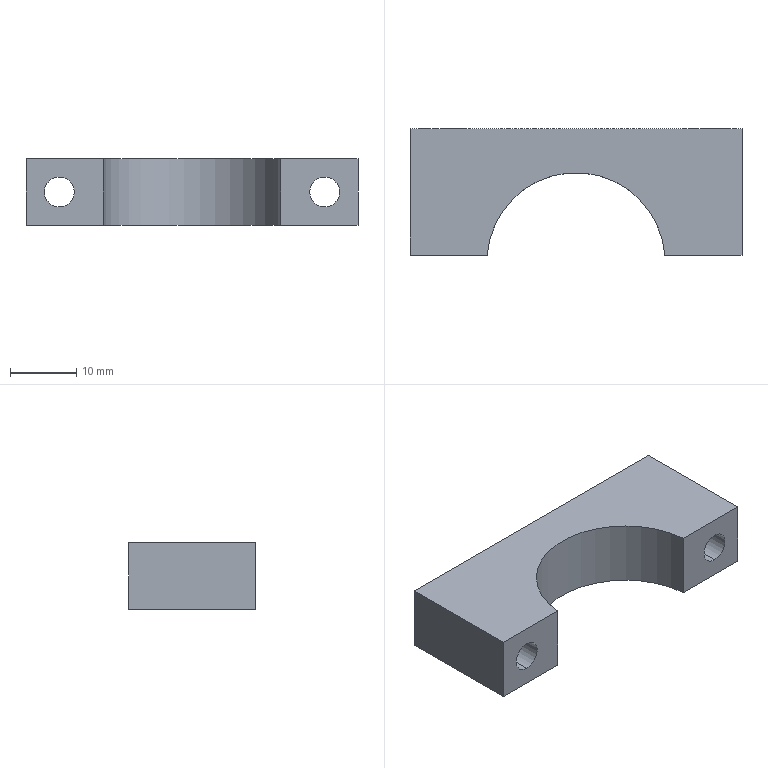Part | STEP file | 2096 Bag feed cylinder support plate B | 1 solid | 18 faces | box 50 x 19 x 10 mm | volume 6027 mm3 | cylinder 9 | plane 9 | commonest cylinder face diameters 4.5 x4 8 x4 26.8 x1
STEP:
#1=CARTESIAN_POINT('',(0.,0.,0.));
#2=DIRECTION('',(0.,0.,1.));
#3=DIRECTION('',(1.,0.,0.));
#4=AXIS2_PLACEMENT_3D('',#1,#2,#3);
#5=CARTESIAN_POINT('',(-20.,5.4,9.));
#6=VERTEX_POINT('',#5);
#7=CARTESIAN_POINT('',(-20.,10.,9.));
#8=VERTEX_POINT('',#7);
#9=CARTESIAN_POINT('',(-20.,10.,9.));
#10=DIRECTION('',(0.,1.,0.));
#11=VECTOR('',#10,1.);
#12=LINE('',#9,#11);
#13=CARTESIAN_POINT('',(-20.,10.,5.));
#14=DIRECTION('',(0.,1.,0.));
#15=DIRECTION('',(0.,0.,1.));
#16=AXIS2_PLACEMENT_3D('',#13,#14,#15);
#17=CYLINDRICAL_SURFACE('',#16,4.);
#18=CARTESIAN_POINT('',(6.283,0.));
#19=DIRECTION('',(0.,1.));
#20=VECTOR('',#19,1.);
#21=LINE('',#18,#20);
#22=(GEOMETRIC_REPRESENTATION_CONTEXT(2)PARAMETRIC_REPRESENTATION_CONTEXT()REPRESENTATION_CONTEXT('',''));
#23=DEFINITIONAL_REPRESENTATION('',(#21),#22);
#24=PCURVE('',#17,#23);
#25=CARTESIAN_POINT('',(-20.,10.,5.));
#26=DIRECTION('',(0.,1.,0.));
#27=DIRECTION('',(0.,0.,1.));
#28=AXIS2_PLACEMENT_3D('',#25,#26,#27);
#29=CYLINDRICAL_SURFACE('',#28,4.);
#30=CARTESIAN_POINT('',(0.,0.));
#31=DIRECTION('',(0.,1.));
#32=VECTOR('',#31,1.);
#33=LINE('',#30,#32);
#34=(GEOMETRIC_REPRESENTATION_CONTEXT(2)PARAMETRIC_REPRESENTATION_CONTEXT()REPRESENTATION_CONTEXT('',''));
#35=DEFINITIONAL_REPRESENTATION('',(#33),#34);
#36=PCURVE('',#29,#35);
#37=SURFACE_CURVE('',#12,(#24,#36),.PCURVE_S1.);
#38=EDGE_CURVE('',#6,#8,#37,.T.);
#39=ORIENTED_EDGE('',*,*,#38,.T.);
#40=CARTESIAN_POINT('',(-20.,10.,1.));
#41=VERTEX_POINT('',#40);
#42=CARTESIAN_POINT('',(-20.,10.,5.));
#43=DIRECTION('',(0.,1.,0.));
#44=DIRECTION('',(0.,0.,1.));
#45=AXIS2_PLACEMENT_3D('',#42,#43,#44);
#46=CIRCLE('',#45,4.);
#47=CARTESIAN_POINT('',(0.,0.));
#48=DIRECTION('',(1.,0.));
#49=VECTOR('',#48,1.);
#50=LINE('',#47,#49);
#51=(GEOMETRIC_REPRESENTATION_CONTEXT(2)PARAMETRIC_REPRESENTATION_CONTEXT()REPRESENTATION_CONTEXT('',''));
#52=DEFINITIONAL_REPRESENTATION('',(#50),#51);
#53=PCURVE('',#17,#52);
#54=CARTESIAN_POINT('',(-25.,10.,10.));
#55=DIRECTION('',(0.,-1.,0.));
#56=DIRECTION('',(0.,0.,-1.));
#57=AXIS2_PLACEMENT_3D('',#54,#55,#56);
#58=PLANE('',#57);
#59=CARTESIAN_POINT('',(1.,5.));
#60=CARTESIAN_POINT('',(1.,11.928));
#61=CARTESIAN_POINT('',(7.,8.464));
#62=CARTESIAN_POINT('',(13.,5.));
#63=CARTESIAN_POINT('',(7.,1.536));
#64=CARTESIAN_POINT('',(1.,-1.928));
#65=CARTESIAN_POINT('',(1.,5.));
#66=(BOUNDED_CURVE()B_SPLINE_CURVE(2,(#59,#60,#61,#62,#63,#64,#65),.UNSPECIFIED.,.T.,.F.)B_SPLINE_CURVE_WITH_KNOTS((1,2,2,2,2,1),(-2.094,0.,2.094,4.189,6.283,8.378),.UNSPECIFIED.)CURVE()GEOMETRIC_REPRESENTATION_ITEM()RATIONAL_B_SPLINE_CURVE((1.,0.5,1.,0.5,1.,0.5,1.))REPRESENTATION_ITEM(''));
#67=(GEOMETRIC_REPRESENTATION_CONTEXT(2)PARAMETRIC_REPRESENTATION_CONTEXT()REPRESENTATION_CONTEXT('',''));
#68=DEFINITIONAL_REPRESENTATION('',(#66),#67);
#69=PCURVE('',#58,#68);
#70=SURFACE_CURVE('',#46,(#53,#69),.PCURVE_S1.);
#71=EDGE_CURVE('',#41,#8,#70,.T.);
#72=ORIENTED_EDGE('',*,*,#71,.F.);
#73=CARTESIAN_POINT('',(-20.,5.4,1.));
#74=VERTEX_POINT('',#73);
#75=CARTESIAN_POINT('',(-20.,10.,1.));
#76=DIRECTION('',(0.,1.,0.));
#77=VECTOR('',#76,1.);
#78=LINE('',#75,#77);
#79=CARTESIAN_POINT('',(3.142,0.));
#80=DIRECTION('',(0.,1.));
#81=VECTOR('',#80,1.);
#82=LINE('',#79,#81);
#83=(GEOMETRIC_REPRESENTATION_CONTEXT(2)PARAMETRIC_REPRESENTATION_CONTEXT()REPRESENTATION_CONTEXT('',''));
#84=DEFINITIONAL_REPRESENTATION('',(#82),#83);
#85=PCURVE('',#17,#84);
#86=CARTESIAN_POINT('',(3.142,0.));
#87=DIRECTION('',(0.,1.));
#88=VECTOR('',#87,1.);
#89=LINE('',#86,#88);
#90=(GEOMETRIC_REPRESENTATION_CONTEXT(2)PARAMETRIC_REPRESENTATION_CONTEXT()REPRESENTATION_CONTEXT('',''));
#91=DEFINITIONAL_REPRESENTATION('',(#89),#90);
#92=PCURVE('',#29,#91);
#93=SURFACE_CURVE('',#78,(#85,#92),.PCURVE_S1.);
#94=EDGE_CURVE('',#74,#41,#93,.T.);
#95=ORIENTED_EDGE('',*,*,#94,.F.);
#96=CARTESIAN_POINT('',(-20.,5.4,5.));
#97=DIRECTION('',(0.,1.,0.));
#98=DIRECTION('',(0.,0.,1.));
#99=AXIS2_PLACEMENT_3D('',#96,#97,#98);
#100=CIRCLE('',#99,4.);
#101=CARTESIAN_POINT('',(0.,-4.6));
#102=DIRECTION('',(1.,0.));
#103=VECTOR('',#102,1.);
#104=LINE('',#101,#103);
#105=(GEOMETRIC_REPRESENTATION_CONTEXT(2)PARAMETRIC_REPRESENTATION_CONTEXT()REPRESENTATION_CONTEXT('',''));
#106=DEFINITIONAL_REPRESENTATION('',(#104),#105);
#107=PCURVE('',#17,#106);
#108=CARTESIAN_POINT('',(-17.75,5.4,5.));
#109=DIRECTION('',(0.,-1.,0.));
#110=DIRECTION('',(0.,0.,-1.));
#111=AXIS2_PLACEMENT_3D('',#108,#109,#110);
#112=PLANE('',#111);
#113=CARTESIAN_POINT('',(-4.,-2.25));
#114=CARTESIAN_POINT('',(-4.,4.678));
#115=CARTESIAN_POINT('',(2.,1.214));
#116=CARTESIAN_POINT('',(8.,-2.25));
#117=CARTESIAN_POINT('',(2.,-5.714));
#118=CARTESIAN_POINT('',(-4.,-9.178));
#119=CARTESIAN_POINT('',(-4.,-2.25));
#120=(BOUNDED_CURVE()B_SPLINE_CURVE(2,(#113,#114,#115,#116,#117,#118,#119),.UNSPECIFIED.,.T.,.F.)B_SPLINE_CURVE_WITH_KNOTS((1,2,2,2,2,1),(-2.094,0.,2.094,4.189,6.283,8.378),.UNSPECIFIED.)CURVE()GEOMETRIC_REPRESENTATION_ITEM()RATIONAL_B_SPLINE_CURVE((1.,0.5,1.,0.5,1.,0.5,1.))REPRESENTATION_ITEM(''));
#121=(GEOMETRIC_REPRESENTATION_CONTEXT(2)PARAMETRIC_REPRESENTATION_CONTEXT()REPRESENTATION_CONTEXT('',''));
#122=DEFINITIONAL_REPRESENTATION('',(#120),#121);
#123=PCURVE('',#112,#122);
#124=SURFACE_CURVE('',#100,(#107,#123),.PCURVE_S1.);
#125=EDGE_CURVE('',#74,#6,#124,.T.);
#126=ORIENTED_EDGE('',*,*,#125,.T.);
#127=EDGE_LOOP('',(#39,#72,#95,#126));
#128=FACE_BOUND('',#127,.F.);
#129=ADVANCED_FACE('',(#128),#17,.F.);
#130=CARTESIAN_POINT('',(-20.,-9.,7.25));
#131=VERTEX_POINT('',#130);
#132=CARTESIAN_POINT('',(-20.,5.4,7.25));
#133=VERTEX_POINT('',#132);
#134=CARTESIAN_POINT('',(-20.,10.,7.25));
#135=DIRECTION('',(0.,1.,0.));
#136=VECTOR('',#135,1.);
#137=LINE('',#134,#136);
#138=CARTESIAN_POINT('',(-20.,10.,5.));
#139=DIRECTION('',(0.,1.,0.));
#140=DIRECTION('',(0.,0.,1.));
#141=AXIS2_PLACEMENT_3D('',#138,#139,#140);
#142=CYLINDRICAL_SURFACE('',#141,2.25);
#143=CARTESIAN_POINT('',(6.283,0.));
#144=DIRECTION('',(0.,1.));
#145=VECTOR('',#144,1.);
#146=LINE('',#143,#145);
#147=(GEOMETRIC_REPRESENTATION_CONTEXT(2)PARAMETRIC_REPRESENTATION_CONTEXT()REPRESENTATION_CONTEXT('',''));
#148=DEFINITIONAL_REPRESENTATION('',(#146),#147);
#149=PCURVE('',#142,#148);
#150=CARTESIAN_POINT('',(-20.,10.,5.));
#151=DIRECTION('',(0.,1.,0.));
#152=DIRECTION('',(0.,0.,1.));
#153=AXIS2_PLACEMENT_3D('',#150,#151,#152);
#154=CYLINDRICAL_SURFACE('',#153,2.25);
#155=CARTESIAN_POINT('',(0.,0.));
#156=DIRECTION('',(0.,1.));
#157=VECTOR('',#156,1.);
#158=LINE('',#155,#157);
#159=(GEOMETRIC_REPRESENTATION_CONTEXT(2)PARAMETRIC_REPRESENTATION_CONTEXT()REPRESENTATION_CONTEXT('',''));
#160=DEFINITIONAL_REPRESENTATION('',(#158),#159);
#161=PCURVE('',#154,#160);
#162=SURFACE_CURVE('',#137,(#149,#161),.PCURVE_S1.);
#163=EDGE_CURVE('',#131,#133,#162,.T.);
#164=ORIENTED_EDGE('',*,*,#163,.T.);
#165=CARTESIAN_POINT('',(-20.,5.4,2.75));
#166=VERTEX_POINT('',#165);
#167=CARTESIAN_POINT('',(-20.,5.4,5.));
#168=DIRECTION('',(0.,1.,0.));
#169=DIRECTION('',(0.,0.,1.));
#170=AXIS2_PLACEMENT_3D('',#167,#168,#169);
#171=CIRCLE('',#170,2.25);
#172=CARTESIAN_POINT('',(0.,-4.6));
#173=DIRECTION('',(1.,0.));
#174=VECTOR('',#173,1.);
#175=LINE('',#172,#174);
#176=(GEOMETRIC_REPRESENTATION_CONTEXT(2)PARAMETRIC_REPRESENTATION_CONTEXT()REPRESENTATION_CONTEXT('',''));
#177=DEFINITIONAL_REPRESENTATION('',(#175),#176);
#178=PCURVE('',#142,#177);
#179=CARTESIAN_POINT('',(-2.25,-2.25));
#180=CARTESIAN_POINT('',(-2.25,1.647));
#181=CARTESIAN_POINT('',(1.125,-0.3014));
#182=CARTESIAN_POINT('',(4.5,-2.25));
#183=CARTESIAN_POINT('',(1.125,-4.199));
#184=CARTESIAN_POINT('',(-2.25,-6.147));
#185=CARTESIAN_POINT('',(-2.25,-2.25));
#186=(BOUNDED_CURVE()B_SPLINE_CURVE(2,(#179,#180,#181,#182,#183,#184,#185),.UNSPECIFIED.,.T.,.F.)B_SPLINE_CURVE_WITH_KNOTS((1,2,2,2,2,1),(-2.094,0.,2.094,4.189,6.283,8.378),.UNSPECIFIED.)CURVE()GEOMETRIC_REPRESENTATION_ITEM()RATIONAL_B_SPLINE_CURVE((1.,0.5,1.,0.5,1.,0.5,1.))REPRESENTATION_ITEM(''));
#187=(GEOMETRIC_REPRESENTATION_CONTEXT(2)PARAMETRIC_REPRESENTATION_CONTEXT()REPRESENTATION_CONTEXT('',''));
#188=DEFINITIONAL_REPRESENTATION('',(#186),#187);
#189=PCURVE('',#112,#188);
#190=SURFACE_CURVE('',#171,(#178,#189),.PCURVE_S1.);
#191=EDGE_CURVE('',#166,#133,#190,.T.);
#192=ORIENTED_EDGE('',*,*,#191,.F.);
#193=CARTESIAN_POINT('',(-20.,-9.,2.75));
#194=VERTEX_POINT('',#193);
#195=CARTESIAN_POINT('',(-20.,10.,2.75));
#196=DIRECTION('',(0.,1.,0.));
#197=VECTOR('',#196,1.);
#198=LINE('',#195,#197);
#199=CARTESIAN_POINT('',(3.142,0.));
#200=DIRECTION('',(0.,1.));
#201=VECTOR('',#200,1.);
#202=LINE('',#199,#201);
#203=(GEOMETRIC_REPRESENTATION_CONTEXT(2)PARAMETRIC_REPRESENTATION_CONTEXT()REPRESENTATION_CONTEXT('',''));
#204=DEFINITIONAL_REPRESENTATION('',(#202),#203);
#205=PCURVE('',#142,#204);
#206=CARTESIAN_POINT('',(3.142,0.));
#207=DIRECTION('',(0.,1.));
#208=VECTOR('',#207,1.);
#209=LINE('',#206,#208);
#210=(GEOMETRIC_REPRESENTATION_CONTEXT(2)PARAMETRIC_REPRESENTATION_CONTEXT()REPRESENTATION_CONTEXT('',''));
#211=DEFINITIONAL_REPRESENTATION('',(#209),#210);
#212=PCURVE('',#154,#211);
#213=SURFACE_CURVE('',#198,(#205,#212),.PCURVE_S1.);
#214=EDGE_CURVE('',#194,#166,#213,.T.);
#215=ORIENTED_EDGE('',*,*,#214,.F.);
#216=CARTESIAN_POINT('',(-20.,-9.,5.));
#217=DIRECTION('',(0.,-1.,0.));
#218=DIRECTION('',(0.,0.,1.));
#219=AXIS2_PLACEMENT_3D('',#216,#217,#218);
#220=CIRCLE('',#219,2.25);
#221=CARTESIAN_POINT('',(6.283,-19.));
#222=DIRECTION('',(-1.,0.));
#223=VECTOR('',#222,1.);
#224=LINE('',#221,#223);
#225=(GEOMETRIC_REPRESENTATION_CONTEXT(2)PARAMETRIC_REPRESENTATION_CONTEXT()REPRESENTATION_CONTEXT('',''));
#226=DEFINITIONAL_REPRESENTATION('',(#224),#225);
#227=PCURVE('',#142,#226);
#228=CARTESIAN_POINT('',(-25.,-9.,0.));
#229=DIRECTION('',(0.,1.,0.));
#230=DIRECTION('',(0.,0.,1.));
#231=AXIS2_PLACEMENT_3D('',#228,#229,#230);
#232=PLANE('',#231);
#233=CARTESIAN_POINT('',(7.25,5.));
#234=CARTESIAN_POINT('',(7.25,1.103));
#235=CARTESIAN_POINT('',(3.875,3.051));
#236=CARTESIAN_POINT('',(0.5,5.));
#237=CARTESIAN_POINT('',(3.875,6.949));
#238=CARTESIAN_POINT('',(7.25,8.897));
#239=CARTESIAN_POINT('',(7.25,5.));
#240=(BOUNDED_CURVE()B_SPLINE_CURVE(2,(#233,#234,#235,#236,#237,#238,#239),.UNSPECIFIED.,.T.,.F.)B_SPLINE_CURVE_WITH_KNOTS((1,2,2,2,2,1),(-2.094,0.,2.094,4.189,6.283,8.378),.UNSPECIFIED.)CURVE()GEOMETRIC_REPRESENTATION_ITEM()RATIONAL_B_SPLINE_CURVE((1.,0.5,1.,0.5,1.,0.5,1.))REPRESENTATION_ITEM(''));
#241=(GEOMETRIC_REPRESENTATION_CONTEXT(2)PARAMETRIC_REPRESENTATION_CONTEXT()REPRESENTATION_CONTEXT('',''));
#242=DEFINITIONAL_REPRESENTATION('',(#240),#241);
#243=PCURVE('',#232,#242);
#244=SURFACE_CURVE('',#220,(#227,#243),.PCURVE_S1.);
#245=EDGE_CURVE('',#131,#194,#244,.T.);
#246=ORIENTED_EDGE('',*,*,#245,.F.);
#247=EDGE_LOOP('',(#164,#192,#215,#246));
#248=FACE_BOUND('',#247,.F.);
#249=ADVANCED_FACE('',(#248),#142,.F.);
#250=CARTESIAN_POINT('',(20.,5.4,9.));
#251=VERTEX_POINT('',#250);
#252=CARTESIAN_POINT('',(20.,10.,9.));
#253=VERTEX_POINT('',#252);
#254=CARTESIAN_POINT('',(20.,10.,9.));
#255=DIRECTION('',(0.,1.,0.));
#256=VECTOR('',#255,1.);
#257=LINE('',#254,#256);
#258=CARTESIAN_POINT('',(20.,10.,5.));
#259=DIRECTION('',(0.,1.,0.));
#260=DIRECTION('',(0.,0.,1.));
#261=AXIS2_PLACEMENT_3D('',#258,#259,#260);
#262=CYLINDRICAL_SURFACE('',#261,4.);
#263=CARTESIAN_POINT('',(6.283,0.));
#264=DIRECTION('',(0.,1.));
#265=VECTOR('',#264,1.);
#266=LINE('',#263,#265);
#267=(GEOMETRIC_REPRESENTATION_CONTEXT(2)PARAMETRIC_REPRESENTATION_CONTEXT()REPRESENTATION_CONTEXT('',''));
#268=DEFINITIONAL_REPRESENTATION('',(#266),#267);
#269=PCURVE('',#262,#268);
#270=CARTESIAN_POINT('',(20.,10.,5.));
#271=DIRECTION('',(0.,1.,0.));
#272=DIRECTION('',(0.,0.,1.));
#273=AXIS2_PLACEMENT_3D('',#270,#271,#272);
#274=CYLINDRICAL_SURFACE('',#273,4.);
#275=CARTESIAN_POINT('',(0.,0.));
#276=DIRECTION('',(0.,1.));
#277=VECTOR('',#276,1.);
#278=LINE('',#275,#277);
#279=(GEOMETRIC_REPRESENTATION_CONTEXT(2)PARAMETRIC_REPRESENTATION_CONTEXT()REPRESENTATION_CONTEXT('',''));
#280=DEFINITIONAL_REPRESENTATION('',(#278),#279);
#281=PCURVE('',#274,#280);
#282=SURFACE_CURVE('',#257,(#269,#281),.PCURVE_S1.);
#283=EDGE_CURVE('',#251,#253,#282,.T.);
#284=ORIENTED_EDGE('',*,*,#283,.T.);
#285=CARTESIAN_POINT('',(20.,10.,1.));
#286=VERTEX_POINT('',#285);
#287=CARTESIAN_POINT('',(20.,10.,5.));
#288=DIRECTION('',(0.,1.,0.));
#289=DIRECTION('',(0.,0.,1.));
#290=AXIS2_PLACEMENT_3D('',#287,#288,#289);
#291=CIRCLE('',#290,4.);
#292=CARTESIAN_POINT('',(0.,0.));
#293=DIRECTION('',(1.,0.));
#294=VECTOR('',#293,1.);
#295=LINE('',#292,#294);
#296=(GEOMETRIC_REPRESENTATION_CONTEXT(2)PARAMETRIC_REPRESENTATION_CONTEXT()REPRESENTATION_CONTEXT('',''));
#297=DEFINITIONAL_REPRESENTATION('',(#295),#296);
#298=PCURVE('',#262,#297);
#299=CARTESIAN_POINT('',(1.,45.));
#300=CARTESIAN_POINT('',(1.,51.928));
#301=CARTESIAN_POINT('',(7.,48.464));
#302=CARTESIAN_POINT('',(13.,45.));
#303=CARTESIAN_POINT('',(7.,41.536));
#304=CARTESIAN_POINT('',(1.,38.072));
#305=CARTESIAN_POINT('',(1.,45.));
#306=(BOUNDED_CURVE()B_SPLINE_CURVE(2,(#299,#300,#301,#302,#303,#304,#305),.UNSPECIFIED.,.T.,.F.)B_SPLINE_CURVE_WITH_KNOTS((1,2,2,2,2,1),(-2.094,0.,2.094,4.189,6.283,8.378),.UNSPECIFIED.)CURVE()GEOMETRIC_REPRESENTATION_ITEM()RATIONAL_B_SPLINE_CURVE((1.,0.5,1.,0.5,1.,0.5,1.))REPRESENTATION_ITEM(''));
#307=(GEOMETRIC_REPRESENTATION_CONTEXT(2)PARAMETRIC_REPRESENTATION_CONTEXT()REPRESENTATION_CONTEXT('',''));
#308=DEFINITIONAL_REPRESENTATION('',(#306),#307);
#309=PCURVE('',#58,#308);
#310=SURFACE_CURVE('',#291,(#298,#309),.PCURVE_S1.);
#311=EDGE_CURVE('',#286,#253,#310,.T.);
#312=ORIENTED_EDGE('',*,*,#311,.F.);
#313=CARTESIAN_POINT('',(20.,5.4,1.));
#314=VERTEX_POINT('',#313);
#315=CARTESIAN_POINT('',(20.,10.,1.));
#316=DIRECTION('',(0.,1.,0.));
#317=VECTOR('',#316,1.);
#318=LINE('',#315,#317);
#319=CARTESIAN_POINT('',(3.142,0.));
#320=DIRECTION('',(0.,1.));
#321=VECTOR('',#320,1.);
#322=LINE('',#319,#321);
#323=(GEOMETRIC_REPRESENTATION_CONTEXT(2)PARAMETRIC_REPRESENTATION_CONTEXT()REPRESENTATION_CONTEXT('',''));
#324=DEFINITIONAL_REPRESENTATION('',(#322),#323);
#325=PCURVE('',#262,#324);
#326=CARTESIAN_POINT('',(3.142,0.));
#327=DIRECTION('',(0.,1.));
#328=VECTOR('',#327,1.);
#329=LINE('',#326,#328);
#330=(GEOMETRIC_REPRESENTATION_CONTEXT(2)PARAMETRIC_REPRESENTATION_CONTEXT()REPRESENTATION_CONTEXT('',''));
#331=DEFINITIONAL_REPRESENTATION('',(#329),#330);
#332=PCURVE('',#274,#331);
#333=SURFACE_CURVE('',#318,(#325,#332),.PCURVE_S1.);
#334=EDGE_CURVE('',#314,#286,#333,.T.);
#335=ORIENTED_EDGE('',*,*,#334,.F.);
#336=CARTESIAN_POINT('',(20.,5.4,5.));
#337=DIRECTION('',(0.,1.,0.));
#338=DIRECTION('',(0.,0.,1.));
#339=AXIS2_PLACEMENT_3D('',#336,#337,#338);
#340=CIRCLE('',#339,4.);
#341=CARTESIAN_POINT('',(0.,-4.6));
#342=DIRECTION('',(1.,0.));
#343=VECTOR('',#342,1.);
#344=LINE('',#341,#343);
#345=(GEOMETRIC_REPRESENTATION_CONTEXT(2)PARAMETRIC_REPRESENTATION_CONTEXT()REPRESENTATION_CONTEXT('',''));
#346=DEFINITIONAL_REPRESENTATION('',(#344),#345);
#347=PCURVE('',#262,#346);
#348=CARTESIAN_POINT('',(22.25,5.4,5.));
#349=DIRECTION('',(0.,-1.,0.));
#350=DIRECTION('',(0.,0.,-1.));
#351=AXIS2_PLACEMENT_3D('',#348,#349,#350);
#352=PLANE('',#351);
#353=CARTESIAN_POINT('',(-4.,-2.25));
#354=CARTESIAN_POINT('',(-4.,4.678));
#355=CARTESIAN_POINT('',(2.,1.214));
#356=CARTESIAN_POINT('',(8.,-2.25));
#357=CARTESIAN_POINT('',(2.,-5.714));
#358=CARTESIAN_POINT('',(-4.,-9.178));
#359=CARTESIAN_POINT('',(-4.,-2.25));
#360=(BOUNDED_CURVE()B_SPLINE_CURVE(2,(#353,#354,#355,#356,#357,#358,#359),.UNSPECIFIED.,.T.,.F.)B_SPLINE_CURVE_WITH_KNOTS((1,2,2,2,2,1),(-2.094,0.,2.094,4.189,6.283,8.378),.UNSPECIFIED.)CURVE()GEOMETRIC_REPRESENTATION_ITEM()RATIONAL_B_SPLINE_CURVE((1.,0.5,1.,0.5,1.,0.5,1.))REPRESENTATION_ITEM(''));
#361=(GEOMETRIC_REPRESENTATION_CONTEXT(2)PARAMETRIC_REPRESENTATION_CONTEXT()REPRESENTATION_CONTEXT('',''));
#362=DEFINITIONAL_REPRESENTATION('',(#360),#361);
#363=PCURVE('',#352,#362);
#364=SURFACE_CURVE('',#340,(#347,#363),.PCURVE_S1.);
#365=EDGE_CURVE('',#314,#251,#364,.T.);
#366=ORIENTED_EDGE('',*,*,#365,.T.);
#367=EDGE_LOOP('',(#284,#312,#335,#366));
#368=FACE_BOUND('',#367,.F.);
#369=ADVANCED_FACE('',(#368),#262,.F.);
#370=CARTESIAN_POINT('',(20.,-9.,7.25));
#371=VERTEX_POINT('',#370);
#372=CARTESIAN_POINT('',(20.,5.4,7.25));
#373=VERTEX_POINT('',#372);
#374=CARTESIAN_POINT('',(20.,10.,7.25));
#375=DIRECTION('',(0.,1.,0.));
#376=VECTOR('',#375,1.);
#377=LINE('',#374,#376);
#378=CARTESIAN_POINT('',(20.,10.,5.));
#379=DIRECTION('',(0.,1.,0.));
#380=DIRECTION('',(0.,0.,1.));
#381=AXIS2_PLACEMENT_3D('',#378,#379,#380);
#382=CYLINDRICAL_SURFACE('',#381,2.25);
#383=CARTESIAN_POINT('',(6.283,0.));
#384=DIRECTION('',(0.,1.));
#385=VECTOR('',#384,1.);
#386=LINE('',#383,#385);
#387=(GEOMETRIC_REPRESENTATION_CONTEXT(2)PARAMETRIC_REPRESENTATION_CONTEXT()REPRESENTATION_CONTEXT('',''));
#388=DEFINITIONAL_REPRESENTATION('',(#386),#387);
#389=PCURVE('',#382,#388);
#390=CARTESIAN_POINT('',(20.,10.,5.));
#391=DIRECTION('',(0.,1.,0.));
#392=DIRECTION('',(0.,0.,1.));
#393=AXIS2_PLACEMENT_3D('',#390,#391,#392);
#394=CYLINDRICAL_SURFACE('',#393,2.25);
#395=CARTESIAN_POINT('',(0.,0.));
#396=DIRECTION('',(0.,1.));
#397=VECTOR('',#396,1.);
#398=LINE('',#395,#397);
#399=(GEOMETRIC_REPRESENTATION_CONTEXT(2)PARAMETRIC_REPRESENTATION_CONTEXT()REPRESENTATION_CONTEXT('',''));
#400=DEFINITIONAL_REPRESENTATION('',(#398),#399);
#401=PCURVE('',#394,#400);
#402=SURFACE_CURVE('',#377,(#389,#401),.PCURVE_S1.);
#403=EDGE_CURVE('',#371,#373,#402,.T.);
#404=ORIENTED_EDGE('',*,*,#403,.T.);
#405=CARTESIAN_POINT('',(20.,5.4,2.75));
#406=VERTEX_POINT('',#405);
#407=CARTESIAN_POINT('',(20.,5.4,5.));
#408=DIRECTION('',(0.,1.,0.));
#409=DIRECTION('',(0.,0.,1.));
#410=AXIS2_PLACEMENT_3D('',#407,#408,#409);
#411=CIRCLE('',#410,2.25);
#412=CARTESIAN_POINT('',(0.,-4.6));
#413=DIRECTION('',(1.,0.));
#414=VECTOR('',#413,1.);
#415=LINE('',#412,#414);
#416=(GEOMETRIC_REPRESENTATION_CONTEXT(2)PARAMETRIC_REPRESENTATION_CONTEXT()REPRESENTATION_CONTEXT('',''));
#417=DEFINITIONAL_REPRESENTATION('',(#415),#416);
#418=PCURVE('',#382,#417);
#419=CARTESIAN_POINT('',(-2.25,-2.25));
#420=CARTESIAN_POINT('',(-2.25,1.647));
#421=CARTESIAN_POINT('',(1.125,-0.3014));
#422=CARTESIAN_POINT('',(4.5,-2.25));
#423=CARTESIAN_POINT('',(1.125,-4.199));
#424=CARTESIAN_POINT('',(-2.25,-6.147));
#425=CARTESIAN_POINT('',(-2.25,-2.25));
#426=(BOUNDED_CURVE()B_SPLINE_CURVE(2,(#419,#420,#421,#422,#423,#424,#425),.UNSPECIFIED.,.T.,.F.)B_SPLINE_CURVE_WITH_KNOTS((1,2,2,2,2,1),(-2.094,0.,2.094,4.189,6.283,8.378),.UNSPECIFIED.)CURVE()GEOMETRIC_REPRESENTATION_ITEM()RATIONAL_B_SPLINE_CURVE((1.,0.5,1.,0.5,1.,0.5,1.))REPRESENTATION_ITEM(''));
#427=(GEOMETRIC_REPRESENTATION_CONTEXT(2)PARAMETRIC_REPRESENTATION_CONTEXT()REPRESENTATION_CONTEXT('',''));
#428=DEFINITIONAL_REPRESENTATION('',(#426),#427);
#429=PCURVE('',#352,#428);
#430=SURFACE_CURVE('',#411,(#418,#429),.PCURVE_S1.);
#431=EDGE_CURVE('',#406,#373,#430,.T.);
#432=ORIENTED_EDGE('',*,*,#431,.F.);
#433=CARTESIAN_POINT('',(20.,-9.,2.75));
#434=VERTEX_POINT('',#433);
#435=CARTESIAN_POINT('',(20.,10.,2.75));
#436=DIRECTION('',(0.,1.,0.));
#437=VECTOR('',#436,1.);
#438=LINE('',#435,#437);
#439=CARTESIAN_POINT('',(3.142,0.));
#440=DIRECTION('',(0.,1.));
#441=VECTOR('',#440,1.);
#442=LINE('',#439,#441);
#443=(GEOMETRIC_REPRESENTATION_CONTEXT(2)PARAMETRIC_REPRESENTATION_CONTEXT()REPRESENTATION_CONTEXT('',''));
#444=DEFINITIONAL_REPRESENTATION('',(#442),#443);
#445=PCURVE('',#382,#444);
#446=CARTESIAN_POINT('',(3.142,0.));
#447=DIRECTION('',(0.,1.));
#448=VECTOR('',#447,1.);
#449=LINE('',#446,#448);
#450=(GEOMETRIC_REPRESENTATION_CONTEXT(2)PARAMETRIC_REPRESENTATION_CONTEXT()REPRESENTATION_CONTEXT('',''));
#451=DEFINITIONAL_REPRESENTATION('',(#449),#450);
#452=PCURVE('',#394,#451);
#453=SURFACE_CURVE('',#438,(#445,#452),.PCURVE_S1.);
#454=EDGE_CURVE('',#434,#406,#453,.T.);
#455=ORIENTED_EDGE('',*,*,#454,.F.);
#456=CARTESIAN_POINT('',(20.,-9.,5.));
#457=DIRECTION('',(0.,-1.,0.));
#458=DIRECTION('',(0.,0.,1.));
#459=AXIS2_PLACEMENT_3D('',#456,#457,#458);
#460=CIRCLE('',#459,2.25);
#461=CARTESIAN_POINT('',(6.283,-19.));
#462=DIRECTION('',(-1.,0.));
#463=VECTOR('',#462,1.);
#464=LINE('',#461,#463);
#465=(GEOMETRIC_REPRESENTATION_CONTEXT(2)PARAMETRIC_REPRESENTATION_CONTEXT()REPRESENTATION_CONTEXT('',''));
#466=DEFINITIONAL_REPRESENTATION('',(#464),#465);
#467=PCURVE('',#382,#466);
#468=CARTESIAN_POINT('',(-25.,-9.,0.));
#469=DIRECTION('',(0.,1.,0.));
#470=DIRECTION('',(0.,0.,1.));
#471=AXIS2_PLACEMENT_3D('',#468,#469,#470);
#472=PLANE('',#471);
#473=CARTESIAN_POINT('',(7.25,45.));
#474=CARTESIAN_POINT('',(7.25,41.103));
#475=CARTESIAN_POINT('',(3.875,43.051));
#476=CARTESIAN_POINT('',(0.5,45.));
#477=CARTESIAN_POINT('',(3.875,46.949));
#478=CARTESIAN_POINT('',(7.25,48.897));
#479=CARTESIAN_POINT('',(7.25,45.));
#480=(BOUNDED_CURVE()B_SPLINE_CURVE(2,(#473,#474,#475,#476,#477,#478,#479),.UNSPECIFIED.,.T.,.F.)B_SPLINE_CURVE_WITH_KNOTS((1,2,2,2,2,1),(-2.094,0.,2.094,4.189,6.283,8.378),.UNSPECIFIED.)CURVE()GEOMETRIC_REPRESENTATION_ITEM()RATIONAL_B_SPLINE_CURVE((1.,0.5,1.,0.5,1.,0.5,1.))REPRESENTATION_ITEM(''));
#481=(GEOMETRIC_REPRESENTATION_CONTEXT(2)PARAMETRIC_REPRESENTATION_CONTEXT()REPRESENTATION_CONTEXT('',''));
#482=DEFINITIONAL_REPRESENTATION('',(#480),#481);
#483=PCURVE('',#472,#482);
#484=SURFACE_CURVE('',#460,(#467,#483),.PCURVE_S1.);
#485=EDGE_CURVE('',#371,#434,#484,.T.);
#486=ORIENTED_EDGE('',*,*,#485,.F.);
#487=EDGE_LOOP('',(#404,#432,#455,#486));
#488=FACE_BOUND('',#487,.F.);
#489=ADVANCED_FACE('',(#488),#382,.F.);
#490=CARTESIAN_POINT('',(25.,-9.,10.));
#491=VERTEX_POINT('',#490);
#492=CARTESIAN_POINT('',(25.,10.,10.));
#493=VERTEX_POINT('',#492);
#494=CARTESIAN_POINT('',(25.,-10.,10.));
#495=DIRECTION('',(0.,1.,0.));
#496=VECTOR('',#495,1.);
#497=LINE('',#494,#496);
#498=CARTESIAN_POINT('',(25.,-10.,10.));
#499=DIRECTION('',(-1.,0.,0.));
#500=DIRECTION('',(0.,0.,1.));
#501=AXIS2_PLACEMENT_3D('',#498,#499,#500);
#502=PLANE('',#501);
#503=CARTESIAN_POINT('',(0.,0.));
#504=DIRECTION('',(0.,1.));
#505=VECTOR('',#504,1.);
#506=LINE('',#503,#505);
#507=(GEOMETRIC_REPRESENTATION_CONTEXT(2)PARAMETRIC_REPRESENTATION_CONTEXT()REPRESENTATION_CONTEXT('',''));
#508=DEFINITIONAL_REPRESENTATION('',(#506),#507);
#509=PCURVE('',#502,#508);
#510=CARTESIAN_POINT('',(0.,0.,10.));
#511=DIRECTION('',(0.,0.,-1.));
#512=DIRECTION('',(-1.,0.,0.));
#513=AXIS2_PLACEMENT_3D('',#510,#511,#512);
#514=PLANE('',#513);
#515=CARTESIAN_POINT('',(-25.,-10.));
#516=DIRECTION('',(0.,1.));
#517=VECTOR('',#516,1.);
#518=LINE('',#515,#517);
#519=(GEOMETRIC_REPRESENTATION_CONTEXT(2)PARAMETRIC_REPRESENTATION_CONTEXT()REPRESENTATION_CONTEXT('',''));
#520=DEFINITIONAL_REPRESENTATION('',(#518),#519);
#521=PCURVE('',#514,#520);
#522=SURFACE_CURVE('',#497,(#509,#521),.PCURVE_S1.);
#523=EDGE_CURVE('',#491,#493,#522,.T.);
#524=ORIENTED_EDGE('',*,*,#523,.F.);
#525=CARTESIAN_POINT('',(25.,-9.,0.));
#526=VERTEX_POINT('',#525);
#527=CARTESIAN_POINT('',(25.,-9.,0.));
#528=DIRECTION('',(0.,0.,1.));
#529=VECTOR('',#528,1.);
#530=LINE('',#527,#529);
#531=CARTESIAN_POINT('',(-10.,1.));
#532=DIRECTION('',(1.,0.));
#533=VECTOR('',#532,1.);
#534=LINE('',#531,#533);
#535=(GEOMETRIC_REPRESENTATION_CONTEXT(2)PARAMETRIC_REPRESENTATION_CONTEXT()REPRESENTATION_CONTEXT('',''));
#536=DEFINITIONAL_REPRESENTATION('',(#534),#535);
#537=PCURVE('',#502,#536);
#538=CARTESIAN_POINT('',(0.,50.));
#539=DIRECTION('',(1.,0.));
#540=VECTOR('',#539,1.);
#541=LINE('',#538,#540);
#542=(GEOMETRIC_REPRESENTATION_CONTEXT(2)PARAMETRIC_REPRESENTATION_CONTEXT()REPRESENTATION_CONTEXT('',''));
#543=DEFINITIONAL_REPRESENTATION('',(#541),#542);
#544=PCURVE('',#472,#543);
#545=SURFACE_CURVE('',#530,(#537,#544),.PCURVE_S1.);
#546=EDGE_CURVE('',#526,#491,#545,.T.);
#547=ORIENTED_EDGE('',*,*,#546,.F.);
#548=CARTESIAN_POINT('',(25.,10.,0.));
#549=VERTEX_POINT('',#548);
#550=CARTESIAN_POINT('',(25.,-10.,0.));
#551=DIRECTION('',(0.,1.,0.));
#552=VECTOR('',#551,1.);
#553=LINE('',#550,#552);
#554=CARTESIAN_POINT('',(-10.,0.));
#555=DIRECTION('',(0.,1.));
#556=VECTOR('',#555,1.);
#557=LINE('',#554,#556);
#558=(GEOMETRIC_REPRESENTATION_CONTEXT(2)PARAMETRIC_REPRESENTATION_CONTEXT()REPRESENTATION_CONTEXT('',''));
#559=DEFINITIONAL_REPRESENTATION('',(#557),#558);
#560=PCURVE('',#502,#559);
#561=CARTESIAN_POINT('',(0.,0.,0.));
#562=DIRECTION('',(0.,0.,-1.));
#563=DIRECTION('',(-1.,0.,0.));
#564=AXIS2_PLACEMENT_3D('',#561,#562,#563);
#565=PLANE('',#564);
#566=CARTESIAN_POINT('',(-25.,-10.));
#567=DIRECTION('',(0.,1.));
#568=VECTOR('',#567,1.);
#569=LINE('',#566,#568);
#570=(GEOMETRIC_REPRESENTATION_CONTEXT(2)PARAMETRIC_REPRESENTATION_CONTEXT()REPRESENTATION_CONTEXT('',''));
#571=DEFINITIONAL_REPRESENTATION('',(#569),#570);
#572=PCURVE('',#565,#571);
#573=SURFACE_CURVE('',#553,(#560,#572),.PCURVE_S1.);
#574=EDGE_CURVE('',#526,#549,#573,.T.);
#575=ORIENTED_EDGE('',*,*,#574,.T.);
#576=CARTESIAN_POINT('',(25.,10.,10.));
#577=DIRECTION('',(0.,0.,-1.));
#578=VECTOR('',#577,1.);
#579=LINE('',#576,#578);
#580=CARTESIAN_POINT('',(0.,20.));
#581=DIRECTION('',(-1.,0.));
#582=VECTOR('',#581,1.);
#583=LINE('',#580,#582);
#584=(GEOMETRIC_REPRESENTATION_CONTEXT(2)PARAMETRIC_REPRESENTATION_CONTEXT()REPRESENTATION_CONTEXT('',''));
#585=DEFINITIONAL_REPRESENTATION('',(#583),#584);
#586=PCURVE('',#502,#585);
#587=CARTESIAN_POINT('',(0.,50.));
#588=DIRECTION('',(1.,0.));
#589=VECTOR('',#588,1.);
#590=LINE('',#587,#589);
#591=(GEOMETRIC_REPRESENTATION_CONTEXT(2)PARAMETRIC_REPRESENTATION_CONTEXT()REPRESENTATION_CONTEXT('',''));
#592=DEFINITIONAL_REPRESENTATION('',(#590),#591);
#593=PCURVE('',#58,#592);
#594=SURFACE_CURVE('',#579,(#586,#593),.PCURVE_S1.);
#595=EDGE_CURVE('',#493,#549,#594,.T.);
#596=ORIENTED_EDGE('',*,*,#595,.F.);
#597=EDGE_LOOP('',(#524,#547,#575,#596));
#598=FACE_BOUND('',#597,.T.);
#599=ADVANCED_FACE('',(#598),#502,.F.);
#600=CARTESIAN_POINT('',(-20.,10.,5.));
#601=DIRECTION('',(0.,1.,0.));
#602=DIRECTION('',(0.,0.,1.));
#603=AXIS2_PLACEMENT_3D('',#600,#601,#602);
#604=CIRCLE('',#603,4.);
#605=CARTESIAN_POINT('',(1.,5.));
#606=CARTESIAN_POINT('',(1.,11.928));
#607=CARTESIAN_POINT('',(7.,8.464));
#608=CARTESIAN_POINT('',(13.,5.));
#609=CARTESIAN_POINT('',(7.,1.536));
#610=CARTESIAN_POINT('',(1.,-1.928));
#611=CARTESIAN_POINT('',(1.,5.));
#612=(BOUNDED_CURVE()B_SPLINE_CURVE(2,(#605,#606,#607,#608,#609,#610,#611),.UNSPECIFIED.,.T.,.F.)B_SPLINE_CURVE_WITH_KNOTS((1,2,2,2,2,1),(-2.094,0.,2.094,4.189,6.283,8.378),.UNSPECIFIED.)CURVE()GEOMETRIC_REPRESENTATION_ITEM()RATIONAL_B_SPLINE_CURVE((1.,0.5,1.,0.5,1.,0.5,1.))REPRESENTATION_ITEM(''));
#613=(GEOMETRIC_REPRESENTATION_CONTEXT(2)PARAMETRIC_REPRESENTATION_CONTEXT()REPRESENTATION_CONTEXT('',''));
#614=DEFINITIONAL_REPRESENTATION('',(#612),#613);
#615=PCURVE('',#58,#614);
#616=CARTESIAN_POINT('',(0.,0.));
#617=DIRECTION('',(1.,0.));
#618=VECTOR('',#617,1.);
#619=LINE('',#616,#618);
#620=(GEOMETRIC_REPRESENTATION_CONTEXT(2)PARAMETRIC_REPRESENTATION_CONTEXT()REPRESENTATION_CONTEXT('',''));
#621=DEFINITIONAL_REPRESENTATION('',(#619),#620);
#622=PCURVE('',#29,#621);
#623=SURFACE_CURVE('',#604,(#615,#622),.PCURVE_S1.);
#624=EDGE_CURVE('',#8,#41,#623,.T.);
#625=ORIENTED_EDGE('',*,*,#624,.F.);
#626=ORIENTED_EDGE('',*,*,#71,.F.);
#627=EDGE_LOOP('',(#625,#626));
#628=FACE_BOUND('',#627,.T.);
#629=CARTESIAN_POINT('',(20.,10.,5.));
#630=DIRECTION('',(0.,1.,0.));
#631=DIRECTION('',(0.,0.,1.));
#632=AXIS2_PLACEMENT_3D('',#629,#630,#631);
#633=CIRCLE('',#632,4.);
#634=CARTESIAN_POINT('',(1.,45.));
#635=CARTESIAN_POINT('',(1.,51.928));
#636=CARTESIAN_POINT('',(7.,48.464));
#637=CARTESIAN_POINT('',(13.,45.));
#638=CARTESIAN_POINT('',(7.,41.536));
#639=CARTESIAN_POINT('',(1.,38.072));
#640=CARTESIAN_POINT('',(1.,45.));
#641=(BOUNDED_CURVE()B_SPLINE_CURVE(2,(#634,#635,#636,#637,#638,#639,#640),.UNSPECIFIED.,.T.,.F.)B_SPLINE_CURVE_WITH_KNOTS((1,2,2,2,2,1),(-2.094,0.,2.094,4.189,6.283,8.378),.UNSPECIFIED.)CURVE()GEOMETRIC_REPRESENTATION_ITEM()RATIONAL_B_SPLINE_CURVE((1.,0.5,1.,0.5,1.,0.5,1.))REPRESENTATION_ITEM(''));
#642=(GEOMETRIC_REPRESENTATION_CONTEXT(2)PARAMETRIC_REPRESENTATION_CONTEXT()REPRESENTATION_CONTEXT('',''));
#643=DEFINITIONAL_REPRESENTATION('',(#641),#642);
#644=PCURVE('',#58,#643);
#645=CARTESIAN_POINT('',(0.,0.));
#646=DIRECTION('',(1.,0.));
#647=VECTOR('',#646,1.);
#648=LINE('',#645,#647);
#649=(GEOMETRIC_REPRESENTATION_CONTEXT(2)PARAMETRIC_REPRESENTATION_CONTEXT()REPRESENTATION_CONTEXT('',''));
#650=DEFINITIONAL_REPRESENTATION('',(#648),#649);
#651=PCURVE('',#274,#650);
#652=SURFACE_CURVE('',#633,(#644,#651),.PCURVE_S1.);
#653=EDGE_CURVE('',#253,#286,#652,.T.);
#654=ORIENTED_EDGE('',*,*,#653,.F.);
#655=ORIENTED_EDGE('',*,*,#311,.F.);
#656=EDGE_LOOP('',(#654,#655));
#657=FACE_BOUND('',#656,.T.);
#658=CARTESIAN_POINT('',(-25.,10.,0.));
#659=VERTEX_POINT('',#658);
#660=CARTESIAN_POINT('',(-25.,10.,0.));
#661=DIRECTION('',(-1.,0.,0.));
#662=VECTOR('',#661,1.);
#663=LINE('',#660,#662);
#664=CARTESIAN_POINT('',(10.,0.));
#665=DIRECTION('',(0.,-1.));
#666=VECTOR('',#665,1.);
#667=LINE('',#664,#666);
#668=(GEOMETRIC_REPRESENTATION_CONTEXT(2)PARAMETRIC_REPRESENTATION_CONTEXT()REPRESENTATION_CONTEXT('',''));
#669=DEFINITIONAL_REPRESENTATION('',(#667),#668);
#670=PCURVE('',#58,#669);
#671=CARTESIAN_POINT('',(25.,10.));
#672=DIRECTION('',(1.,0.));
#673=VECTOR('',#672,1.);
#674=LINE('',#671,#673);
#675=(GEOMETRIC_REPRESENTATION_CONTEXT(2)PARAMETRIC_REPRESENTATION_CONTEXT()REPRESENTATION_CONTEXT('',''));
#676=DEFINITIONAL_REPRESENTATION('',(#674),#675);
#677=PCURVE('',#565,#676);
#678=SURFACE_CURVE('',#663,(#670,#677),.PCURVE_S1.);
#679=EDGE_CURVE('',#549,#659,#678,.T.);
#680=ORIENTED_EDGE('',*,*,#679,.T.);
#681=CARTESIAN_POINT('',(-25.,10.,10.));
#682=VERTEX_POINT('',#681);
#683=CARTESIAN_POINT('',(-25.,10.,10.));
#684=DIRECTION('',(0.,0.,-1.));
#685=VECTOR('',#684,1.);
#686=LINE('',#683,#685);
#687=CARTESIAN_POINT('',(0.,0.));
#688=DIRECTION('',(1.,0.));
#689=VECTOR('',#688,1.);
#690=LINE('',#687,#689);
#691=(GEOMETRIC_REPRESENTATION_CONTEXT(2)PARAMETRIC_REPRESENTATION_CONTEXT()REPRESENTATION_CONTEXT('',''));
#692=DEFINITIONAL_REPRESENTATION('',(#690),#691);
#693=PCURVE('',#58,#692);
#694=CARTESIAN_POINT('',(-25.,-10.,10.));
#695=DIRECTION('',(1.,0.,0.));
#696=DIRECTION('',(0.,0.,-1.));
#697=AXIS2_PLACEMENT_3D('',#694,#695,#696);
#698=PLANE('',#697);
#699=CARTESIAN_POINT('',(0.,20.));
#700=DIRECTION('',(1.,0.));
#701=VECTOR('',#700,1.);
#702=LINE('',#699,#701);
#703=(GEOMETRIC_REPRESENTATION_CONTEXT(2)PARAMETRIC_REPRESENTATION_CONTEXT()REPRESENTATION_CONTEXT('',''));
#704=DEFINITIONAL_REPRESENTATION('',(#702),#703);
#705=PCURVE('',#698,#704);
#706=SURFACE_CURVE('',#686,(#693,#705),.PCURVE_S1.);
#707=EDGE_CURVE('',#682,#659,#706,.T.);
#708=ORIENTED_EDGE('',*,*,#707,.F.);
#709=CARTESIAN_POINT('',(-25.,10.,10.));
#710=DIRECTION('',(-1.,0.,0.));
#711=VECTOR('',#710,1.);
#712=LINE('',#709,#711);
#713=CARTESIAN_POINT('',(0.,0.));
#714=DIRECTION('',(0.,-1.));
#715=VECTOR('',#714,1.);
#716=LINE('',#713,#715);
#717=(GEOMETRIC_REPRESENTATION_CONTEXT(2)PARAMETRIC_REPRESENTATION_CONTEXT()REPRESENTATION_CONTEXT('',''));
#718=DEFINITIONAL_REPRESENTATION('',(#716),#717);
#719=PCURVE('',#58,#718);
#720=CARTESIAN_POINT('',(25.,10.));
#721=DIRECTION('',(1.,0.));
#722=VECTOR('',#721,1.);
#723=LINE('',#720,#722);
#724=(GEOMETRIC_REPRESENTATION_CONTEXT(2)PARAMETRIC_REPRESENTATION_CONTEXT()REPRESENTATION_CONTEXT('',''));
#725=DEFINITIONAL_REPRESENTATION('',(#723),#724);
#726=PCURVE('',#514,#725);
#727=SURFACE_CURVE('',#712,(#719,#726),.PCURVE_S1.);
#728=EDGE_CURVE('',#493,#682,#727,.T.);
#729=ORIENTED_EDGE('',*,*,#728,.F.);
#730=ORIENTED_EDGE('',*,*,#595,.T.);
#731=EDGE_LOOP('',(#680,#708,#729,#730));
#732=FACE_BOUND('',#731,.T.);
#733=ADVANCED_FACE('',(#628,#657,#732),#58,.F.);
#734=CARTESIAN_POINT('',(-25.,-9.,0.));
#735=VERTEX_POINT('',#734);
#736=CARTESIAN_POINT('',(-25.,-10.,0.));
#737=DIRECTION('',(0.,-1.,0.));
#738=VECTOR('',#737,1.);
#739=LINE('',#736,#738);
#740=CARTESIAN_POINT('',(10.,0.));
#741=DIRECTION('',(0.,-1.));
#742=VECTOR('',#741,1.);
#743=LINE('',#740,#742);
#744=(GEOMETRIC_REPRESENTATION_CONTEXT(2)PARAMETRIC_REPRESENTATION_CONTEXT()REPRESENTATION_CONTEXT('',''));
#745=DEFINITIONAL_REPRESENTATION('',(#743),#744);
#746=PCURVE('',#698,#745);
#747=CARTESIAN_POINT('',(25.,-10.));
#748=DIRECTION('',(0.,-1.));
#749=VECTOR('',#748,1.);
#750=LINE('',#747,#749);
#751=(GEOMETRIC_REPRESENTATION_CONTEXT(2)PARAMETRIC_REPRESENTATION_CONTEXT()REPRESENTATION_CONTEXT('',''));
#752=DEFINITIONAL_REPRESENTATION('',(#750),#751);
#753=PCURVE('',#565,#752);
#754=SURFACE_CURVE('',#739,(#746,#753),.PCURVE_S1.);
#755=EDGE_CURVE('',#659,#735,#754,.T.);
#756=ORIENTED_EDGE('',*,*,#755,.T.);
#757=CARTESIAN_POINT('',(-25.,-9.,10.));
#758=VERTEX_POINT('',#757);
#759=CARTESIAN_POINT('',(-25.,-9.,0.));
#760=DIRECTION('',(0.,0.,1.));
#761=VECTOR('',#760,1.);
#762=LINE('',#759,#761);
#763=CARTESIAN_POINT('',(10.,1.));
#764=DIRECTION('',(-1.,0.));
#765=VECTOR('',#764,1.);
#766=LINE('',#763,#765);
#767=(GEOMETRIC_REPRESENTATION_CONTEXT(2)PARAMETRIC_REPRESENTATION_CONTEXT()REPRESENTATION_CONTEXT('',''));
#768=DEFINITIONAL_REPRESENTATION('',(#766),#767);
#769=PCURVE('',#698,#768);
#770=CARTESIAN_POINT('',(0.,0.));
#771=DIRECTION('',(1.,0.));
#772=VECTOR('',#771,1.);
#773=LINE('',#770,#772);
#774=(GEOMETRIC_REPRESENTATION_CONTEXT(2)PARAMETRIC_REPRESENTATION_CONTEXT()REPRESENTATION_CONTEXT('',''));
#775=DEFINITIONAL_REPRESENTATION('',(#773),#774);
#776=PCURVE('',#232,#775);
#777=SURFACE_CURVE('',#762,(#769,#776),.PCURVE_S1.);
#778=EDGE_CURVE('',#735,#758,#777,.T.);
#779=ORIENTED_EDGE('',*,*,#778,.T.);
#780=CARTESIAN_POINT('',(-25.,-10.,10.));
#781=DIRECTION('',(0.,-1.,0.));
#782=VECTOR('',#781,1.);
#783=LINE('',#780,#782);
#784=CARTESIAN_POINT('',(0.,0.));
#785=DIRECTION('',(0.,-1.));
#786=VECTOR('',#785,1.);
#787=LINE('',#784,#786);
#788=(GEOMETRIC_REPRESENTATION_CONTEXT(2)PARAMETRIC_REPRESENTATION_CONTEXT()REPRESENTATION_CONTEXT('',''));
#789=DEFINITIONAL_REPRESENTATION('',(#787),#788);
#790=PCURVE('',#698,#789);
#791=CARTESIAN_POINT('',(25.,-10.));
#792=DIRECTION('',(0.,-1.));
#793=VECTOR('',#792,1.);
#794=LINE('',#791,#793);
#795=(GEOMETRIC_REPRESENTATION_CONTEXT(2)PARAMETRIC_REPRESENTATION_CONTEXT()REPRESENTATION_CONTEXT('',''));
#796=DEFINITIONAL_REPRESENTATION('',(#794),#795);
#797=PCURVE('',#514,#796);
#798=SURFACE_CURVE('',#783,(#790,#797),.PCURVE_S1.);
#799=EDGE_CURVE('',#682,#758,#798,.T.);
#800=ORIENTED_EDGE('',*,*,#799,.F.);
#801=ORIENTED_EDGE('',*,*,#707,.T.);
#802=EDGE_LOOP('',(#756,#779,#800,#801));
#803=FACE_BOUND('',#802,.T.);
#804=ADVANCED_FACE('',(#803),#698,.F.);
#805=ORIENTED_EDGE('',*,*,#799,.T.);
#806=CARTESIAN_POINT('',(-13.363,-9.,10.));
#807=VERTEX_POINT('',#806);
#808=CARTESIAN_POINT('',(-25.,-9.,10.));
#809=DIRECTION('',(-1.,0.,0.));
#810=VECTOR('',#809,1.);
#811=LINE('',#808,#810);
#812=CARTESIAN_POINT('',(25.,-9.));
#813=DIRECTION('',(1.,0.));
#814=VECTOR('',#813,1.);
#815=LINE('',#812,#814);
#816=(GEOMETRIC_REPRESENTATION_CONTEXT(2)PARAMETRIC_REPRESENTATION_CONTEXT()REPRESENTATION_CONTEXT('',''));
#817=DEFINITIONAL_REPRESENTATION('',(#815),#816);
#818=PCURVE('',#514,#817);
#819=CARTESIAN_POINT('',(10.,0.));
#820=DIRECTION('',(0.,-1.));
#821=VECTOR('',#820,1.);
#822=LINE('',#819,#821);
#823=(GEOMETRIC_REPRESENTATION_CONTEXT(2)PARAMETRIC_REPRESENTATION_CONTEXT()REPRESENTATION_CONTEXT('',''));
#824=DEFINITIONAL_REPRESENTATION('',(#822),#823);
#825=PCURVE('',#232,#824);
#826=SURFACE_CURVE('',#811,(#818,#825),.PCURVE_S1.);
#827=EDGE_CURVE('',#807,#758,#826,.T.);
#828=ORIENTED_EDGE('',*,*,#827,.F.);
#829=CARTESIAN_POINT('',(13.363,-9.,10.));
#830=VERTEX_POINT('',#829);
#831=CARTESIAN_POINT('',(0.,-10.,10.));
#832=DIRECTION('',(0.,0.,1.));
#833=DIRECTION('',(1.,0.,0.));
#834=AXIS2_PLACEMENT_3D('',#831,#832,#833);
#835=CIRCLE('',#834,13.4);
#836=CARTESIAN_POINT('',(-13.4,-10.));
#837=CARTESIAN_POINT('',(-13.4,13.209));
#838=CARTESIAN_POINT('',(6.7,1.605));
#839=CARTESIAN_POINT('',(26.8,-10.));
#840=CARTESIAN_POINT('',(6.7,-21.605));
#841=CARTESIAN_POINT('',(-13.4,-33.209));
#842=CARTESIAN_POINT('',(-13.4,-10.));
#843=(BOUNDED_CURVE()B_SPLINE_CURVE(2,(#836,#837,#838,#839,#840,#841,#842),.UNSPECIFIED.,.T.,.F.)B_SPLINE_CURVE_WITH_KNOTS((1,2,2,2,2,1),(-2.094,0.,2.094,4.189,6.283,8.378),.UNSPECIFIED.)CURVE()GEOMETRIC_REPRESENTATION_ITEM()RATIONAL_B_SPLINE_CURVE((1.,0.5,1.,0.5,1.,0.5,1.))REPRESENTATION_ITEM(''));
#844=(GEOMETRIC_REPRESENTATION_CONTEXT(2)PARAMETRIC_REPRESENTATION_CONTEXT()REPRESENTATION_CONTEXT('',''));
#845=DEFINITIONAL_REPRESENTATION('',(#843),#844);
#846=PCURVE('',#514,#845);
#847=CARTESIAN_POINT('',(0.,-10.,0.));
#848=DIRECTION('',(0.,0.,1.));
#849=DIRECTION('',(1.,0.,0.));
#850=AXIS2_PLACEMENT_3D('',#847,#848,#849);
#851=CYLINDRICAL_SURFACE('',#850,13.4);
#852=CARTESIAN_POINT('',(0.,10.));
#853=DIRECTION('',(1.,0.));
#854=VECTOR('',#853,1.);
#855=LINE('',#852,#854);
#856=(GEOMETRIC_REPRESENTATION_CONTEXT(2)PARAMETRIC_REPRESENTATION_CONTEXT()REPRESENTATION_CONTEXT('',''));
#857=DEFINITIONAL_REPRESENTATION('',(#855),#856);
#858=PCURVE('',#851,#857);
#859=SURFACE_CURVE('',#835,(#846,#858),.PCURVE_S1.);
#860=EDGE_CURVE('',#830,#807,#859,.T.);
#861=ORIENTED_EDGE('',*,*,#860,.F.);
#862=CARTESIAN_POINT('',(-25.,-9.,10.));
#863=DIRECTION('',(-1.,0.,0.));
#864=VECTOR('',#863,1.);
#865=LINE('',#862,#864);
#866=CARTESIAN_POINT('',(25.,-9.));
#867=DIRECTION('',(1.,0.));
#868=VECTOR('',#867,1.);
#869=LINE('',#866,#868);
#870=(GEOMETRIC_REPRESENTATION_CONTEXT(2)PARAMETRIC_REPRESENTATION_CONTEXT()REPRESENTATION_CONTEXT('',''));
#871=DEFINITIONAL_REPRESENTATION('',(#869),#870);
#872=PCURVE('',#514,#871);
#873=CARTESIAN_POINT('',(10.,0.));
#874=DIRECTION('',(0.,-1.));
#875=VECTOR('',#874,1.);
#876=LINE('',#873,#875);
#877=(GEOMETRIC_REPRESENTATION_CONTEXT(2)PARAMETRIC_REPRESENTATION_CONTEXT()REPRESENTATION_CONTEXT('',''));
#878=DEFINITIONAL_REPRESENTATION('',(#876),#877);
#879=PCURVE('',#472,#878);
#880=SURFACE_CURVE('',#865,(#872,#879),.PCURVE_S1.);
#881=EDGE_CURVE('',#491,#830,#880,.T.);
#882=ORIENTED_EDGE('',*,*,#881,.F.);
#883=ORIENTED_EDGE('',*,*,#523,.T.);
#884=ORIENTED_EDGE('',*,*,#728,.T.);
#885=EDGE_LOOP('',(#805,#828,#861,#882,#883,#884));
#886=FACE_BOUND('',#885,.T.);
#887=ADVANCED_FACE('',(#886),#514,.F.);
#888=CARTESIAN_POINT('',(-13.363,-9.,0.));
#889=VERTEX_POINT('',#888);
#890=CARTESIAN_POINT('',(-25.,-9.,0.));
#891=DIRECTION('',(-1.,0.,0.));
#892=VECTOR('',#891,1.);
#893=LINE('',#890,#892);
#894=CARTESIAN_POINT('',(25.,-9.));
#895=DIRECTION('',(1.,0.));
#896=VECTOR('',#895,1.);
#897=LINE('',#894,#896);
#898=(GEOMETRIC_REPRESENTATION_CONTEXT(2)PARAMETRIC_REPRESENTATION_CONTEXT()REPRESENTATION_CONTEXT('',''));
#899=DEFINITIONAL_REPRESENTATION('',(#897),#898);
#900=PCURVE('',#565,#899);
#901=CARTESIAN_POINT('',(0.,0.));
#902=DIRECTION('',(0.,-1.));
#903=VECTOR('',#902,1.);
#904=LINE('',#901,#903);
#905=(GEOMETRIC_REPRESENTATION_CONTEXT(2)PARAMETRIC_REPRESENTATION_CONTEXT()REPRESENTATION_CONTEXT('',''));
#906=DEFINITIONAL_REPRESENTATION('',(#904),#905);
#907=PCURVE('',#232,#906);
#908=SURFACE_CURVE('',#893,(#900,#907),.PCURVE_S1.);
#909=EDGE_CURVE('',#889,#735,#908,.T.);
#910=ORIENTED_EDGE('',*,*,#909,.T.);
#911=ORIENTED_EDGE('',*,*,#755,.F.);
#912=ORIENTED_EDGE('',*,*,#679,.F.);
#913=ORIENTED_EDGE('',*,*,#574,.F.);
#914=CARTESIAN_POINT('',(13.363,-9.,0.));
#915=VERTEX_POINT('',#914);
#916=CARTESIAN_POINT('',(-25.,-9.,0.));
#917=DIRECTION('',(-1.,0.,0.));
#918=VECTOR('',#917,1.);
#919=LINE('',#916,#918);
#920=CARTESIAN_POINT('',(25.,-9.));
#921=DIRECTION('',(1.,0.));
#922=VECTOR('',#921,1.);
#923=LINE('',#920,#922);
#924=(GEOMETRIC_REPRESENTATION_CONTEXT(2)PARAMETRIC_REPRESENTATION_CONTEXT()REPRESENTATION_CONTEXT('',''));
#925=DEFINITIONAL_REPRESENTATION('',(#923),#924);
#926=PCURVE('',#565,#925);
#927=CARTESIAN_POINT('',(0.,0.));
#928=DIRECTION('',(0.,-1.));
#929=VECTOR('',#928,1.);
#930=LINE('',#927,#929);
#931=(GEOMETRIC_REPRESENTATION_CONTEXT(2)PARAMETRIC_REPRESENTATION_CONTEXT()REPRESENTATION_CONTEXT('',''));
#932=DEFINITIONAL_REPRESENTATION('',(#930),#931);
#933=PCURVE('',#472,#932);
#934=SURFACE_CURVE('',#919,(#926,#933),.PCURVE_S1.);
#935=EDGE_CURVE('',#526,#915,#934,.T.);
#936=ORIENTED_EDGE('',*,*,#935,.T.);
#937=CARTESIAN_POINT('',(0.,-10.,0.));
#938=DIRECTION('',(0.,0.,1.));
#939=DIRECTION('',(1.,0.,0.));
#940=AXIS2_PLACEMENT_3D('',#937,#938,#939);
#941=CIRCLE('',#940,13.4);
#942=CARTESIAN_POINT('',(-13.4,-10.));
#943=CARTESIAN_POINT('',(-13.4,13.209));
#944=CARTESIAN_POINT('',(6.7,1.605));
#945=CARTESIAN_POINT('',(26.8,-10.));
#946=CARTESIAN_POINT('',(6.7,-21.605));
#947=CARTESIAN_POINT('',(-13.4,-33.209));
#948=CARTESIAN_POINT('',(-13.4,-10.));
#949=(BOUNDED_CURVE()B_SPLINE_CURVE(2,(#942,#943,#944,#945,#946,#947,#948),.UNSPECIFIED.,.T.,.F.)B_SPLINE_CURVE_WITH_KNOTS((1,2,2,2,2,1),(-2.094,0.,2.094,4.189,6.283,8.378),.UNSPECIFIED.)CURVE()GEOMETRIC_REPRESENTATION_ITEM()RATIONAL_B_SPLINE_CURVE((1.,0.5,1.,0.5,1.,0.5,1.))REPRESENTATION_ITEM(''));
#950=(GEOMETRIC_REPRESENTATION_CONTEXT(2)PARAMETRIC_REPRESENTATION_CONTEXT()REPRESENTATION_CONTEXT('',''));
#951=DEFINITIONAL_REPRESENTATION('',(#949),#950);
#952=PCURVE('',#565,#951);
#953=CARTESIAN_POINT('',(0.,0.));
#954=DIRECTION('',(1.,0.));
#955=VECTOR('',#954,1.);
#956=LINE('',#953,#955);
#957=(GEOMETRIC_REPRESENTATION_CONTEXT(2)PARAMETRIC_REPRESENTATION_CONTEXT()REPRESENTATION_CONTEXT('',''));
#958=DEFINITIONAL_REPRESENTATION('',(#956),#957);
#959=PCURVE('',#851,#958);
#960=SURFACE_CURVE('',#941,(#952,#959),.PCURVE_S1.);
#961=EDGE_CURVE('',#915,#889,#960,.T.);
#962=ORIENTED_EDGE('',*,*,#961,.T.);
#963=EDGE_LOOP('',(#910,#911,#912,#913,#936,#962));
#964=FACE_BOUND('',#963,.T.);
#965=ADVANCED_FACE('',(#964),#565,.T.);
#966=CARTESIAN_POINT('',(13.363,-9.,0.));
#967=DIRECTION('',(0.,0.,1.));
#968=VECTOR('',#967,1.);
#969=LINE('',#966,#968);
#970=CARTESIAN_POINT('',(0.0747,0.));
#971=DIRECTION('',(0.,1.));
#972=VECTOR('',#971,1.);
#973=LINE('',#970,#972);
#974=(GEOMETRIC_REPRESENTATION_CONTEXT(2)PARAMETRIC_REPRESENTATION_CONTEXT()REPRESENTATION_CONTEXT('',''));
#975=DEFINITIONAL_REPRESENTATION('',(#973),#974);
#976=PCURVE('',#851,#975);
#977=CARTESIAN_POINT('',(0.,38.363));
#978=DIRECTION('',(1.,0.));
#979=VECTOR('',#978,1.);
#980=LINE('',#977,#979);
#981=(GEOMETRIC_REPRESENTATION_CONTEXT(2)PARAMETRIC_REPRESENTATION_CONTEXT()REPRESENTATION_CONTEXT('',''));
#982=DEFINITIONAL_REPRESENTATION('',(#980),#981);
#983=PCURVE('',#472,#982);
#984=SURFACE_CURVE('',#969,(#976,#983),.PCURVE_S1.);
#985=EDGE_CURVE('',#915,#830,#984,.T.);
#986=ORIENTED_EDGE('',*,*,#985,.F.);
#987=ORIENTED_EDGE('',*,*,#961,.T.);
#988=CARTESIAN_POINT('',(-13.363,-9.,0.));
#989=DIRECTION('',(0.,0.,-1.));
#990=VECTOR('',#989,1.);
#991=LINE('',#988,#990);
#992=CARTESIAN_POINT('',(3.067,0.));
#993=DIRECTION('',(0.,-1.));
#994=VECTOR('',#993,1.);
#995=LINE('',#992,#994);
#996=(GEOMETRIC_REPRESENTATION_CONTEXT(2)PARAMETRIC_REPRESENTATION_CONTEXT()REPRESENTATION_CONTEXT('',''));
#997=DEFINITIONAL_REPRESENTATION('',(#995),#996);
#998=PCURVE('',#851,#997);
#999=CARTESIAN_POINT('',(0.,11.637));
#1000=DIRECTION('',(-1.,0.));
#1001=VECTOR('',#1000,1.);
#1002=LINE('',#999,#1001);
#1003=(GEOMETRIC_REPRESENTATION_CONTEXT(2)PARAMETRIC_REPRESENTATION_CONTEXT()REPRESENTATION_CONTEXT('',''));
#1004=DEFINITIONAL_REPRESENTATION('',(#1002),#1003);
#1005=PCURVE('',#232,#1004);
#1006=SURFACE_CURVE('',#991,(#998,#1005),.PCURVE_S1.);
#1007=EDGE_CURVE('',#807,#889,#1006,.T.);
#1008=ORIENTED_EDGE('',*,*,#1007,.F.);
#1009=ORIENTED_EDGE('',*,*,#860,.F.);
#1010=EDGE_LOOP('',(#986,#987,#1008,#1009));
#1011=FACE_BOUND('',#1010,.F.);
#1012=ADVANCED_FACE('',(#1011),#851,.F.);
#1013=CARTESIAN_POINT('',(20.,5.4,5.));
#1014=DIRECTION('',(0.,1.,0.));
#1015=DIRECTION('',(0.,0.,1.));
#1016=AXIS2_PLACEMENT_3D('',#1013,#1014,#1015);
#1017=CIRCLE('',#1016,2.25);
#1018=CARTESIAN_POINT('',(0.,-4.6));
#1019=DIRECTION('',(1.,0.));
#1020=VECTOR('',#1019,1.);
#1021=LINE('',#1018,#1020);
#1022=(GEOMETRIC_REPRESENTATION_CONTEXT(2)PARAMETRIC_REPRESENTATION_CONTEXT()REPRESENTATION_CONTEXT('',''));
#1023=DEFINITIONAL_REPRESENTATION('',(#1021),#1022);
#1024=PCURVE('',#394,#1023);
#1025=CARTESIAN_POINT('',(-2.25,-2.25));
#1026=CARTESIAN_POINT('',(-2.25,1.647));
#1027=CARTESIAN_POINT('',(1.125,-0.3014));
#1028=CARTESIAN_POINT('',(4.5,-2.25));
#1029=CARTESIAN_POINT('',(1.125,-4.199));
#1030=CARTESIAN_POINT('',(-2.25,-6.147));
#1031=CARTESIAN_POINT('',(-2.25,-2.25));
#1032=(BOUNDED_CURVE()B_SPLINE_CURVE(2,(#1025,#1026,#1027,#1028,#1029,#1030,#1031),.UNSPECIFIED.,.T.,.F.)B_SPLINE_CURVE_WITH_KNOTS((1,2,2,2,2,1),(-2.094,0.,2.094,4.189,6.283,8.378),.UNSPECIFIED.)CURVE()GEOMETRIC_REPRESENTATION_ITEM()RATIONAL_B_SPLINE_CURVE((1.,0.5,1.,0.5,1.,0.5,1.))REPRESENTATION_ITEM(''));
#1033=(GEOMETRIC_REPRESENTATION_CONTEXT(2)PARAMETRIC_REPRESENTATION_CONTEXT()REPRESENTATION_CONTEXT('',''));
#1034=DEFINITIONAL_REPRESENTATION('',(#1032),#1033);
#1035=PCURVE('',#352,#1034);
#1036=SURFACE_CURVE('',#1017,(#1024,#1035),.PCURVE_S1.);
#1037=EDGE_CURVE('',#373,#406,#1036,.T.);
#1038=ORIENTED_EDGE('',*,*,#1037,.F.);
#1039=ORIENTED_EDGE('',*,*,#403,.F.);
#1040=CARTESIAN_POINT('',(20.,-9.,5.));
#1041=DIRECTION('',(0.,-1.,0.));
#1042=DIRECTION('',(0.,0.,1.));
#1043=AXIS2_PLACEMENT_3D('',#1040,#1041,#1042);
#1044=CIRCLE('',#1043,2.25);
#1045=CARTESIAN_POINT('',(6.283,-19.));
#1046=DIRECTION('',(-1.,0.));
#1047=VECTOR('',#1046,1.);
#1048=LINE('',#1045,#1047);
#1049=(GEOMETRIC_REPRESENTATION_CONTEXT(2)PARAMETRIC_REPRESENTATION_CONTEXT()REPRESENTATION_CONTEXT('',''));
#1050=DEFINITIONAL_REPRESENTATION('',(#1048),#1049);
#1051=PCURVE('',#394,#1050);
#1052=CARTESIAN_POINT('',(7.25,45.));
#1053=CARTESIAN_POINT('',(7.25,41.103));
#1054=CARTESIAN_POINT('',(3.875,43.051));
#1055=CARTESIAN_POINT('',(0.5,45.));
#1056=CARTESIAN_POINT('',(3.875,46.949));
#1057=CARTESIAN_POINT('',(7.25,48.897));
#1058=CARTESIAN_POINT('',(7.25,45.));
#1059=(BOUNDED_CURVE()B_SPLINE_CURVE(2,(#1052,#1053,#1054,#1055,#1056,#1057,#1058),.UNSPECIFIED.,.T.,.F.)B_SPLINE_CURVE_WITH_KNOTS((1,2,2,2,2,1),(-2.094,0.,2.094,4.189,6.283,8.378),.UNSPECIFIED.)CURVE()GEOMETRIC_REPRESENTATION_ITEM()RATIONAL_B_SPLINE_CURVE((1.,0.5,1.,0.5,1.,0.5,1.))REPRESENTATION_ITEM(''));
#1060=(GEOMETRIC_REPRESENTATION_CONTEXT(2)PARAMETRIC_REPRESENTATION_CONTEXT()REPRESENTATION_CONTEXT('',''));
#1061=DEFINITIONAL_REPRESENTATION('',(#1059),#1060);
#1062=PCURVE('',#472,#1061);
#1063=SURFACE_CURVE('',#1044,(#1051,#1062),.PCURVE_S1.);
#1064=EDGE_CURVE('',#434,#371,#1063,.T.);
#1065=ORIENTED_EDGE('',*,*,#1064,.F.);
#1066=ORIENTED_EDGE('',*,*,#454,.T.);
#1067=EDGE_LOOP('',(#1038,#1039,#1065,#1066));
#1068=FACE_BOUND('',#1067,.F.);
#1069=ADVANCED_FACE('',(#1068),#394,.F.);
#1070=ORIENTED_EDGE('',*,*,#1037,.F.);
#1071=ORIENTED_EDGE('',*,*,#431,.F.);
#1072=EDGE_LOOP('',(#1070,#1071));
#1073=FACE_BOUND('',#1072,.T.);
#1074=CARTESIAN_POINT('',(20.,5.4,5.));
#1075=DIRECTION('',(0.,1.,0.));
#1076=DIRECTION('',(0.,0.,1.));
#1077=AXIS2_PLACEMENT_3D('',#1074,#1075,#1076);
#1078=CIRCLE('',#1077,4.);
#1079=CARTESIAN_POINT('',(-4.,-2.25));
#1080=CARTESIAN_POINT('',(-4.,4.678));
#1081=CARTESIAN_POINT('',(2.,1.214));
#1082=CARTESIAN_POINT('',(8.,-2.25));
#1083=CARTESIAN_POINT('',(2.,-5.714));
#1084=CARTESIAN_POINT('',(-4.,-9.178));
#1085=CARTESIAN_POINT('',(-4.,-2.25));
#1086=(BOUNDED_CURVE()B_SPLINE_CURVE(2,(#1079,#1080,#1081,#1082,#1083,#1084,#1085),.UNSPECIFIED.,.T.,.F.)B_SPLINE_CURVE_WITH_KNOTS((1,2,2,2,2,1),(-2.094,0.,2.094,4.189,6.283,8.378),.UNSPECIFIED.)CURVE()GEOMETRIC_REPRESENTATION_ITEM()RATIONAL_B_SPLINE_CURVE((1.,0.5,1.,0.5,1.,0.5,1.))REPRESENTATION_ITEM(''));
#1087=(GEOMETRIC_REPRESENTATION_CONTEXT(2)PARAMETRIC_REPRESENTATION_CONTEXT()REPRESENTATION_CONTEXT('',''));
#1088=DEFINITIONAL_REPRESENTATION('',(#1086),#1087);
#1089=PCURVE('',#352,#1088);
#1090=CARTESIAN_POINT('',(0.,-4.6));
#1091=DIRECTION('',(1.,0.));
#1092=VECTOR('',#1091,1.);
#1093=LINE('',#1090,#1092);
#1094=(GEOMETRIC_REPRESENTATION_CONTEXT(2)PARAMETRIC_REPRESENTATION_CONTEXT()REPRESENTATION_CONTEXT('',''));
#1095=DEFINITIONAL_REPRESENTATION('',(#1093),#1094);
#1096=PCURVE('',#274,#1095);
#1097=SURFACE_CURVE('',#1078,(#1089,#1096),.PCURVE_S1.);
#1098=EDGE_CURVE('',#251,#314,#1097,.T.);
#1099=ORIENTED_EDGE('',*,*,#1098,.T.);
#1100=ORIENTED_EDGE('',*,*,#365,.T.);
#1101=EDGE_LOOP('',(#1099,#1100));
#1102=FACE_BOUND('',#1101,.T.);
#1103=ADVANCED_FACE('',(#1073,#1102),#352,.F.);
#1104=ORIENTED_EDGE('',*,*,#653,.F.);
#1105=ORIENTED_EDGE('',*,*,#283,.F.);
#1106=ORIENTED_EDGE('',*,*,#1098,.T.);
#1107=ORIENTED_EDGE('',*,*,#334,.T.);
#1108=EDGE_LOOP('',(#1104,#1105,#1106,#1107));
#1109=FACE_BOUND('',#1108,.F.);
#1110=ADVANCED_FACE('',(#1109),#274,.F.);
#1111=CARTESIAN_POINT('',(-20.,5.4,5.));
#1112=DIRECTION('',(0.,1.,0.));
#1113=DIRECTION('',(0.,0.,1.));
#1114=AXIS2_PLACEMENT_3D('',#1111,#1112,#1113);
#1115=CIRCLE('',#1114,2.25);
#1116=CARTESIAN_POINT('',(0.,-4.6));
#1117=DIRECTION('',(1.,0.));
#1118=VECTOR('',#1117,1.);
#1119=LINE('',#1116,#1118);
#1120=(GEOMETRIC_REPRESENTATION_CONTEXT(2)PARAMETRIC_REPRESENTATION_CONTEXT()REPRESENTATION_CONTEXT('',''));
#1121=DEFINITIONAL_REPRESENTATION('',(#1119),#1120);
#1122=PCURVE('',#154,#1121);
#1123=CARTESIAN_POINT('',(-2.25,-2.25));
#1124=CARTESIAN_POINT('',(-2.25,1.647));
#1125=CARTESIAN_POINT('',(1.125,-0.3014));
#1126=CARTESIAN_POINT('',(4.5,-2.25));
#1127=CARTESIAN_POINT('',(1.125,-4.199));
#1128=CARTESIAN_POINT('',(-2.25,-6.147));
#1129=CARTESIAN_POINT('',(-2.25,-2.25));
#1130=(BOUNDED_CURVE()B_SPLINE_CURVE(2,(#1123,#1124,#1125,#1126,#1127,#1128,#1129),.UNSPECIFIED.,.T.,.F.)B_SPLINE_CURVE_WITH_KNOTS((1,2,2,2,2,1),(-2.094,0.,2.094,4.189,6.283,8.378),.UNSPECIFIED.)CURVE()GEOMETRIC_REPRESENTATION_ITEM()RATIONAL_B_SPLINE_CURVE((1.,0.5,1.,0.5,1.,0.5,1.))REPRESENTATION_ITEM(''));
#1131=(GEOMETRIC_REPRESENTATION_CONTEXT(2)PARAMETRIC_REPRESENTATION_CONTEXT()REPRESENTATION_CONTEXT('',''));
#1132=DEFINITIONAL_REPRESENTATION('',(#1130),#1131);
#1133=PCURVE('',#112,#1132);
#1134=SURFACE_CURVE('',#1115,(#1122,#1133),.PCURVE_S1.);
#1135=EDGE_CURVE('',#133,#166,#1134,.T.);
#1136=ORIENTED_EDGE('',*,*,#1135,.F.);
#1137=ORIENTED_EDGE('',*,*,#163,.F.);
#1138=CARTESIAN_POINT('',(-20.,-9.,5.));
#1139=DIRECTION('',(0.,-1.,0.));
#1140=DIRECTION('',(0.,0.,1.));
#1141=AXIS2_PLACEMENT_3D('',#1138,#1139,#1140);
#1142=CIRCLE('',#1141,2.25);
#1143=CARTESIAN_POINT('',(6.283,-19.));
#1144=DIRECTION('',(-1.,0.));
#1145=VECTOR('',#1144,1.);
#1146=LINE('',#1143,#1145);
#1147=(GEOMETRIC_REPRESENTATION_CONTEXT(2)PARAMETRIC_REPRESENTATION_CONTEXT()REPRESENTATION_CONTEXT('',''));
#1148=DEFINITIONAL_REPRESENTATION('',(#1146),#1147);
#1149=PCURVE('',#154,#1148);
#1150=CARTESIAN_POINT('',(7.25,5.));
#1151=CARTESIAN_POINT('',(7.25,1.103));
#1152=CARTESIAN_POINT('',(3.875,3.051));
#1153=CARTESIAN_POINT('',(0.5,5.));
#1154=CARTESIAN_POINT('',(3.875,6.949));
#1155=CARTESIAN_POINT('',(7.25,8.897));
#1156=CARTESIAN_POINT('',(7.25,5.));
#1157=(BOUNDED_CURVE()B_SPLINE_CURVE(2,(#1150,#1151,#1152,#1153,#1154,#1155,#1156),.UNSPECIFIED.,.T.,.F.)B_SPLINE_CURVE_WITH_KNOTS((1,2,2,2,2,1),(-2.094,0.,2.094,4.189,6.283,8.378),.UNSPECIFIED.)CURVE()GEOMETRIC_REPRESENTATION_ITEM()RATIONAL_B_SPLINE_CURVE((1.,0.5,1.,0.5,1.,0.5,1.))REPRESENTATION_ITEM(''));
#1158=(GEOMETRIC_REPRESENTATION_CONTEXT(2)PARAMETRIC_REPRESENTATION_CONTEXT()REPRESENTATION_CONTEXT('',''));
#1159=DEFINITIONAL_REPRESENTATION('',(#1157),#1158);
#1160=PCURVE('',#232,#1159);
#1161=SURFACE_CURVE('',#1142,(#1149,#1160),.PCURVE_S1.);
#1162=EDGE_CURVE('',#194,#131,#1161,.T.);
#1163=ORIENTED_EDGE('',*,*,#1162,.F.);
#1164=ORIENTED_EDGE('',*,*,#214,.T.);
#1165=EDGE_LOOP('',(#1136,#1137,#1163,#1164));
#1166=FACE_BOUND('',#1165,.F.);
#1167=ADVANCED_FACE('',(#1166),#154,.F.);
#1168=ORIENTED_EDGE('',*,*,#1135,.F.);
#1169=ORIENTED_EDGE('',*,*,#191,.F.);
#1170=EDGE_LOOP('',(#1168,#1169));
#1171=FACE_BOUND('',#1170,.T.);
#1172=CARTESIAN_POINT('',(-20.,5.4,5.));
#1173=DIRECTION('',(0.,1.,0.));
#1174=DIRECTION('',(0.,0.,1.));
#1175=AXIS2_PLACEMENT_3D('',#1172,#1173,#1174);
#1176=CIRCLE('',#1175,4.);
#1177=CARTESIAN_POINT('',(-4.,-2.25));
#1178=CARTESIAN_POINT('',(-4.,4.678));
#1179=CARTESIAN_POINT('',(2.,1.214));
#1180=CARTESIAN_POINT('',(8.,-2.25));
#1181=CARTESIAN_POINT('',(2.,-5.714));
#1182=CARTESIAN_POINT('',(-4.,-9.178));
#1183=CARTESIAN_POINT('',(-4.,-2.25));
#1184=(BOUNDED_CURVE()B_SPLINE_CURVE(2,(#1177,#1178,#1179,#1180,#1181,#1182,#1183),.UNSPECIFIED.,.T.,.F.)B_SPLINE_CURVE_WITH_KNOTS((1,2,2,2,2,1),(-2.094,0.,2.094,4.189,6.283,8.378),.UNSPECIFIED.)CURVE()GEOMETRIC_REPRESENTATION_ITEM()RATIONAL_B_SPLINE_CURVE((1.,0.5,1.,0.5,1.,0.5,1.))REPRESENTATION_ITEM(''));
#1185=(GEOMETRIC_REPRESENTATION_CONTEXT(2)PARAMETRIC_REPRESENTATION_CONTEXT()REPRESENTATION_CONTEXT('',''));
#1186=DEFINITIONAL_REPRESENTATION('',(#1184),#1185);
#1187=PCURVE('',#112,#1186);
#1188=CARTESIAN_POINT('',(0.,-4.6));
#1189=DIRECTION('',(1.,0.));
#1190=VECTOR('',#1189,1.);
#1191=LINE('',#1188,#1190);
#1192=(GEOMETRIC_REPRESENTATION_CONTEXT(2)PARAMETRIC_REPRESENTATION_CONTEXT()REPRESENTATION_CONTEXT('',''));
#1193=DEFINITIONAL_REPRESENTATION('',(#1191),#1192);
#1194=PCURVE('',#29,#1193);
#1195=SURFACE_CURVE('',#1176,(#1187,#1194),.PCURVE_S1.);
#1196=EDGE_CURVE('',#6,#74,#1195,.T.);
#1197=ORIENTED_EDGE('',*,*,#1196,.T.);
#1198=ORIENTED_EDGE('',*,*,#125,.T.);
#1199=EDGE_LOOP('',(#1197,#1198));
#1200=FACE_BOUND('',#1199,.T.);
#1201=ADVANCED_FACE('',(#1171,#1200),#112,.F.);
#1202=ORIENTED_EDGE('',*,*,#624,.F.);
#1203=ORIENTED_EDGE('',*,*,#38,.F.);
#1204=ORIENTED_EDGE('',*,*,#1196,.T.);
#1205=ORIENTED_EDGE('',*,*,#94,.T.);
#1206=EDGE_LOOP('',(#1202,#1203,#1204,#1205));
#1207=FACE_BOUND('',#1206,.F.);
#1208=ADVANCED_FACE('',(#1207),#29,.F.);
#1209=ORIENTED_EDGE('',*,*,#245,.F.);
#1210=ORIENTED_EDGE('',*,*,#1162,.F.);
#1211=EDGE_LOOP('',(#1209,#1210));
#1212=FACE_BOUND('',#1211,.T.);
#1213=ORIENTED_EDGE('',*,*,#827,.T.);
#1214=ORIENTED_EDGE('',*,*,#778,.F.);
#1215=ORIENTED_EDGE('',*,*,#909,.F.);
#1216=ORIENTED_EDGE('',*,*,#1007,.F.);
#1217=EDGE_LOOP('',(#1213,#1214,#1215,#1216));
#1218=FACE_BOUND('',#1217,.T.);
#1219=ADVANCED_FACE('',(#1212,#1218),#232,.F.);
#1220=ORIENTED_EDGE('',*,*,#485,.F.);
#1221=ORIENTED_EDGE('',*,*,#1064,.F.);
#1222=EDGE_LOOP('',(#1220,#1221));
#1223=FACE_BOUND('',#1222,.T.);
#1224=ORIENTED_EDGE('',*,*,#935,.F.);
#1225=ORIENTED_EDGE('',*,*,#546,.T.);
#1226=ORIENTED_EDGE('',*,*,#881,.T.);
#1227=ORIENTED_EDGE('',*,*,#985,.F.);
#1228=EDGE_LOOP('',(#1224,#1225,#1226,#1227));
#1229=FACE_BOUND('',#1228,.T.);
#1230=ADVANCED_FACE('',(#1223,#1229),#472,.F.);
#1231=CLOSED_SHELL('',(#129,#249,#369,#489,#599,#733,#804,#887,#965,#1012,#1069,#1103,#1110,#1167,#1201,#1208,#1219,#1230));
#1232=MANIFOLD_SOLID_BREP('',#1231);
#1233=(LENGTH_UNIT()NAMED_UNIT(*)SI_UNIT(.MILLI.,.METRE.));
#1234=UNCERTAINTY_MEASURE_WITH_UNIT(LENGTH_MEASURE(0.0000001),#1233,'','');
#1235=(NAMED_UNIT(*)PLANE_ANGLE_UNIT()SI_UNIT($,.RADIAN.));
#1236=(NAMED_UNIT(*)SI_UNIT($,.STERADIAN.)SOLID_ANGLE_UNIT());
#1237=(GEOMETRIC_REPRESENTATION_CONTEXT(3)GLOBAL_UNCERTAINTY_ASSIGNED_CONTEXT((#1234))GLOBAL_UNIT_ASSIGNED_CONTEXT((#1233,#1235,#1236))REPRESENTATION_CONTEXT('',''));
#1238=ADVANCED_BREP_SHAPE_REPRESENTATION('',(#4,#1232),#1237);